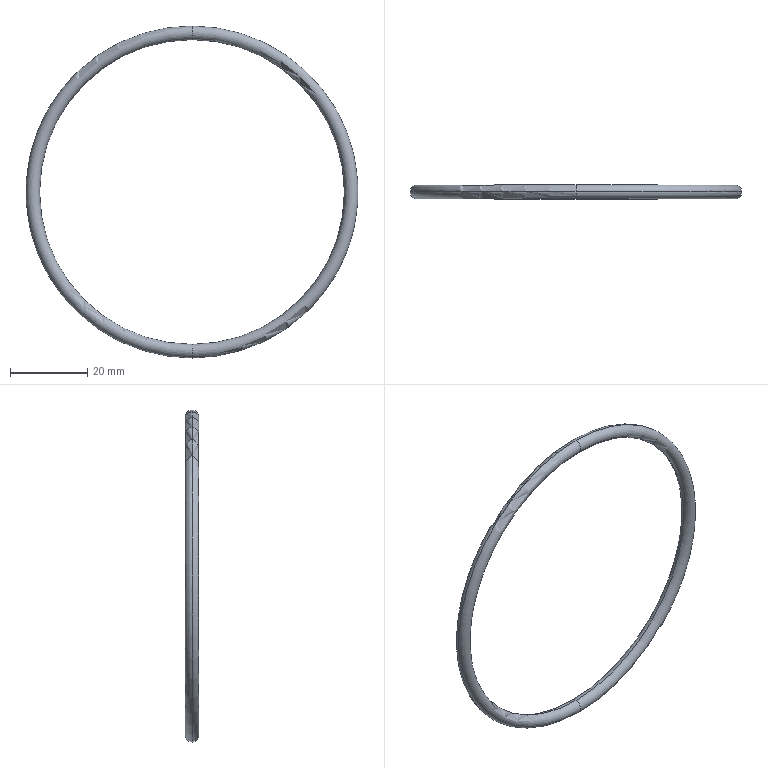Part | SolidWorks | features RefAxis 1, Revolution 1 | 1 solid | 4 faces | box 86.03 x 3.53 x 86.03 mm | volume 2537 mm3 | torus 4
STEP:
#1=CARTESIAN_POINT('',(0.,0.,-43.015));
#2=VERTEX_POINT('',#1);
#3=CARTESIAN_POINT('',(0.,0.,-39.485));
#4=VERTEX_POINT('',#3);
#5=CARTESIAN_POINT('',(0.,0.,-41.25));
#6=DIRECTION('',(1.,0.,0.));
#7=DIRECTION('',(0.,0.,-1.));
#8=AXIS2_PLACEMENT_3D('',#5,#6,#7);
#9=CIRCLE('',#8,1.765);
#10=EDGE_CURVE('',#2,#4,#9,.T.);
#11=ORIENTED_EDGE('',*,*,#10,.F.);
#12=CARTESIAN_POINT('',(0.,0.,43.015));
#13=VERTEX_POINT('',#12);
#14=CARTESIAN_POINT('',(0.,0.,0.));
#15=DIRECTION('',(0.,1.,0.));
#16=DIRECTION('',(0.,0.,1.));
#17=AXIS2_PLACEMENT_3D('',#14,#15,#16);
#18=CIRCLE('',#17,43.015);
#19=EDGE_CURVE('',#2,#13,#18,.T.);
#20=ORIENTED_EDGE('',*,*,#19,.T.);
#21=CARTESIAN_POINT('',(0.,0.,39.485));
#22=VERTEX_POINT('',#21);
#23=CARTESIAN_POINT('',(0.,0.,41.25));
#24=DIRECTION('',(-1.,0.,0.));
#25=DIRECTION('',(0.,0.,1.));
#26=AXIS2_PLACEMENT_3D('',#23,#24,#25);
#27=CIRCLE('',#26,1.765);
#28=EDGE_CURVE('',#13,#22,#27,.T.);
#29=ORIENTED_EDGE('',*,*,#28,.T.);
#30=CARTESIAN_POINT('',(0.,0.,0.));
#31=DIRECTION('',(0.,1.,0.));
#32=DIRECTION('',(0.,0.,1.));
#33=AXIS2_PLACEMENT_3D('',#30,#31,#32);
#34=CIRCLE('',#33,39.485);
#35=EDGE_CURVE('',#4,#22,#34,.T.);
#36=ORIENTED_EDGE('',*,*,#35,.F.);
#37=EDGE_LOOP('',(#11,#20,#29,#36));
#38=FACE_OUTER_BOUND('',#37,.T.);
#39=CARTESIAN_POINT('',(0.,0.,0.));
#40=DIRECTION('',(0.,1.,0.));
#41=DIRECTION('',(0.,0.,1.));
#42=AXIS2_PLACEMENT_3D('',#39,#40,#41);
#43=TOROIDAL_SURFACE('',#42,41.25,1.765);
#44=ADVANCED_FACE('',(#38),#43,.T.);
#45=ORIENTED_EDGE('',*,*,#28,.F.);
#46=CARTESIAN_POINT('',(0.,0.,0.));
#47=DIRECTION('',(0.,1.,0.));
#48=DIRECTION('',(0.,0.,1.));
#49=AXIS2_PLACEMENT_3D('',#46,#47,#48);
#50=CIRCLE('',#49,43.015);
#51=EDGE_CURVE('',#13,#2,#50,.T.);
#52=ORIENTED_EDGE('',*,*,#51,.T.);
#53=ORIENTED_EDGE('',*,*,#10,.T.);
#54=CARTESIAN_POINT('',(0.,0.,0.));
#55=DIRECTION('',(0.,1.,0.));
#56=DIRECTION('',(0.,0.,1.));
#57=AXIS2_PLACEMENT_3D('',#54,#55,#56);
#58=CIRCLE('',#57,39.485);
#59=EDGE_CURVE('',#22,#4,#58,.T.);
#60=ORIENTED_EDGE('',*,*,#59,.F.);
#61=EDGE_LOOP('',(#45,#52,#53,#60));
#62=FACE_OUTER_BOUND('',#61,.T.);
#63=CARTESIAN_POINT('',(0.,0.,0.));
#64=DIRECTION('',(0.,1.,0.));
#65=DIRECTION('',(0.,0.,1.));
#66=AXIS2_PLACEMENT_3D('',#63,#64,#65);
#67=TOROIDAL_SURFACE('',#66,41.25,1.765);
#68=ADVANCED_FACE('',(#62),#67,.T.);
#69=ORIENTED_EDGE('',*,*,#51,.F.);
#70=CARTESIAN_POINT('',(0.,0.,41.25));
#71=DIRECTION('',(-1.,0.,0.));
#72=DIRECTION('',(0.,0.,1.));
#73=AXIS2_PLACEMENT_3D('',#70,#71,#72);
#74=CIRCLE('',#73,1.765);
#75=EDGE_CURVE('',#22,#13,#74,.T.);
#76=ORIENTED_EDGE('',*,*,#75,.F.);
#77=ORIENTED_EDGE('',*,*,#59,.T.);
#78=CARTESIAN_POINT('',(0.,0.,-41.25));
#79=DIRECTION('',(1.,0.,0.));
#80=DIRECTION('',(0.,0.,-1.));
#81=AXIS2_PLACEMENT_3D('',#78,#79,#80);
#82=CIRCLE('',#81,1.765);
#83=EDGE_CURVE('',#4,#2,#82,.T.);
#84=ORIENTED_EDGE('',*,*,#83,.T.);
#85=EDGE_LOOP('',(#69,#76,#77,#84));
#86=FACE_OUTER_BOUND('',#85,.T.);
#87=CARTESIAN_POINT('',(0.,0.,0.));
#88=DIRECTION('',(0.,1.,0.));
#89=DIRECTION('',(0.,0.,1.));
#90=AXIS2_PLACEMENT_3D('',#87,#88,#89);
#91=TOROIDAL_SURFACE('',#90,41.25,1.765);
#92=ADVANCED_FACE('',(#86),#91,.T.);
#93=ORIENTED_EDGE('',*,*,#19,.F.);
#94=ORIENTED_EDGE('',*,*,#83,.F.);
#95=ORIENTED_EDGE('',*,*,#35,.T.);
#96=ORIENTED_EDGE('',*,*,#75,.T.);
#97=EDGE_LOOP('',(#93,#94,#95,#96));
#98=FACE_OUTER_BOUND('',#97,.T.);
#99=CARTESIAN_POINT('',(0.,0.,0.));
#100=DIRECTION('',(0.,1.,0.));
#101=DIRECTION('',(0.,0.,1.));
#102=AXIS2_PLACEMENT_3D('',#99,#100,#101);
#103=TOROIDAL_SURFACE('',#102,41.25,1.765);
#104=ADVANCED_FACE('',(#98),#103,.T.);
#105=CLOSED_SHELL('',(#44,#68,#92,#104));
#106=MANIFOLD_SOLID_BREP('',#105);
#107=CARTESIAN_POINT('',(0.,0.,0.));
#108=DIRECTION('',(0.,0.,1.));
#109=DIRECTION('',(1.,0.,0.));
#110=AXIS2_PLACEMENT_3D('',#107,#108,#109);
#111=(LENGTH_UNIT()NAMED_UNIT(*)SI_UNIT(.MILLI.,.METRE.));
#112=UNCERTAINTY_MEASURE_WITH_UNIT(LENGTH_MEASURE(0.00001),#111,'','');
#113=(NAMED_UNIT(*)PLANE_ANGLE_UNIT()SI_UNIT($,.RADIAN.));
#114=(NAMED_UNIT(*)SI_UNIT($,.STERADIAN.)SOLID_ANGLE_UNIT());
#115=(GEOMETRIC_REPRESENTATION_CONTEXT(3)GLOBAL_UNCERTAINTY_ASSIGNED_CONTEXT((#112))GLOBAL_UNIT_ASSIGNED_CONTEXT((#111,#113,#114))REPRESENTATION_CONTEXT('',''));
#116=ADVANCED_BREP_SHAPE_REPRESENTATION('',(#106,#110),#115);